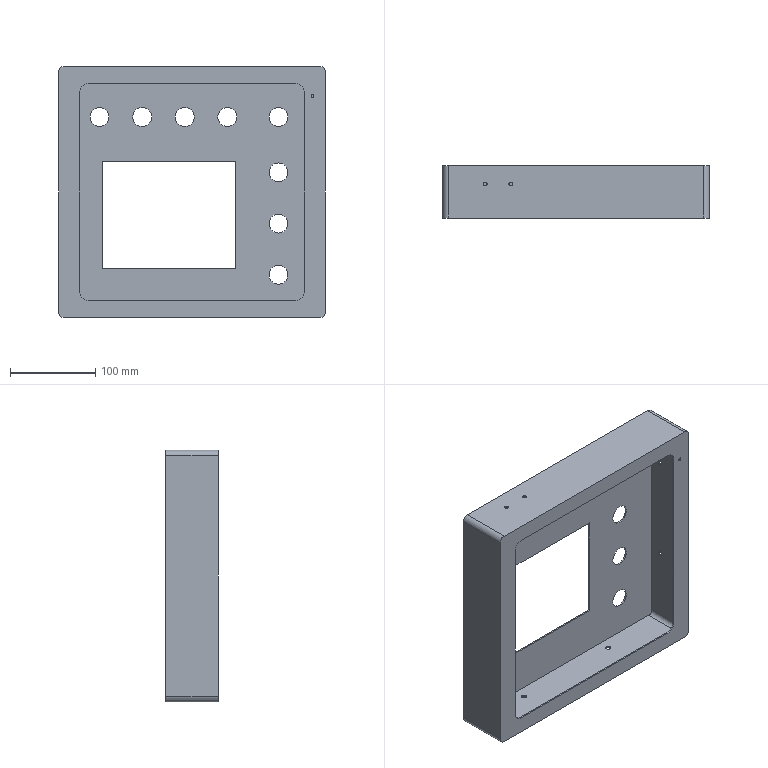Part | STEP file | 227H056120A Front Panel | 1 solid | 62 faces | box 313 x 61.6 x 295 mm | volume 263384 mm3 | cylinder 42 | plane 20 | commonest cylinder face diameters 22.3 x16 6 x8 4.5 x4 10 x4 13.2 x4 20 x4